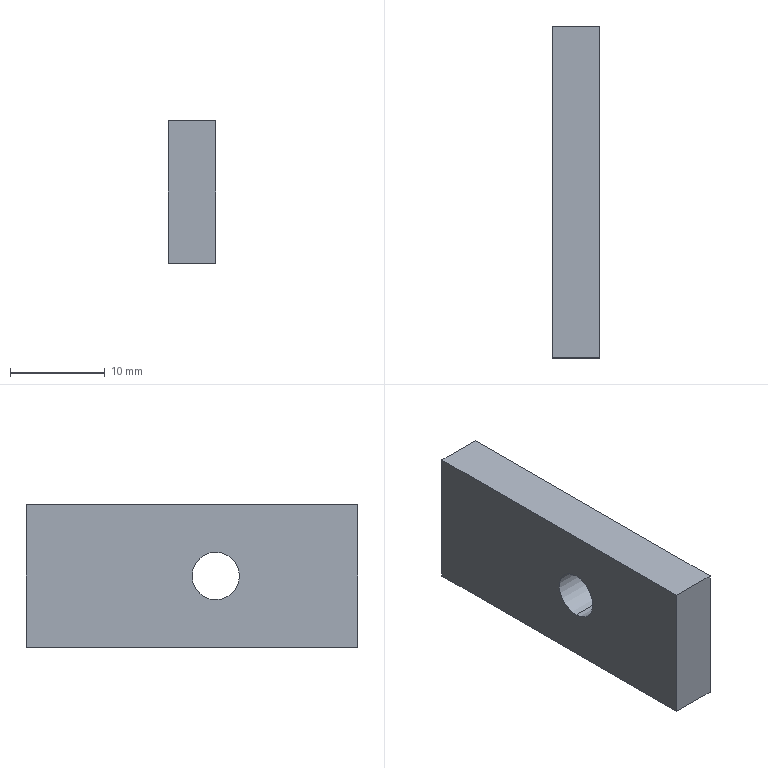Part | SolidWorks | features MBimport 1 | 1 solid | 8 faces | box 5 x 35 x 15 mm | volume 2527 mm3 | plane 6 | cylinder 2 | commonest cylinder face diameters 5 x2
STEP:
#1=CARTESIAN_POINT('',(0.,-15.,7.5));
#2=VERTEX_POINT('',#1);
#3=CARTESIAN_POINT('',(0.,-15.,-7.5));
#4=VERTEX_POINT('',#3);
#5=CARTESIAN_POINT('',(0.,-15.,7.5));
#6=DIRECTION('',(0.,0.,-1.));
#7=VECTOR('',#6,1000.);
#8=LINE('',#5,#7);
#9=EDGE_CURVE('',#2,#4,#8,.T.);
#10=ORIENTED_EDGE('',*,*,#9,.F.);
#11=CARTESIAN_POINT('',(0.,20.,7.5));
#12=VERTEX_POINT('',#11);
#13=CARTESIAN_POINT('',(0.,-15.,7.5));
#14=DIRECTION('',(0.,1.,0.));
#15=VECTOR('',#14,1000.);
#16=LINE('',#13,#15);
#17=EDGE_CURVE('',#2,#12,#16,.T.);
#18=ORIENTED_EDGE('',*,*,#17,.T.);
#19=CARTESIAN_POINT('',(0.,20.,-7.5));
#20=VERTEX_POINT('',#19);
#21=CARTESIAN_POINT('',(0.,20.,-7.5));
#22=DIRECTION('',(0.,0.,1.));
#23=VECTOR('',#22,1000.);
#24=LINE('',#21,#23);
#25=EDGE_CURVE('',#20,#12,#24,.T.);
#26=ORIENTED_EDGE('',*,*,#25,.F.);
#27=CARTESIAN_POINT('',(0.,20.,-7.5));
#28=DIRECTION('',(0.,-1.,0.));
#29=VECTOR('',#28,1000.);
#30=LINE('',#27,#29);
#31=EDGE_CURVE('',#20,#4,#30,.T.);
#32=ORIENTED_EDGE('',*,*,#31,.T.);
#33=EDGE_LOOP('',(#10,#18,#26,#32));
#34=FACE_OUTER_BOUND('',#33,.T.);
#35=CARTESIAN_POINT('',(0.,0.,2.5));
#36=VERTEX_POINT('',#35);
#37=CARTESIAN_POINT('',(0.,0.,-2.5));
#38=VERTEX_POINT('',#37);
#39=CARTESIAN_POINT('',(0.,0.,0.));
#40=DIRECTION('',(1.,0.,0.));
#41=DIRECTION('',(0.,0.,1.));
#42=AXIS2_PLACEMENT_3D('',#39,#40,#41);
#43=CIRCLE('',#42,2.5);
#44=EDGE_CURVE('',#36,#38,#43,.T.);
#45=ORIENTED_EDGE('',*,*,#44,.T.);
#46=CARTESIAN_POINT('',(0.,0.,0.));
#47=DIRECTION('',(1.,0.,0.));
#48=DIRECTION('',(0.,0.,-1.));
#49=AXIS2_PLACEMENT_3D('',#46,#47,#48);
#50=CIRCLE('',#49,2.5);
#51=EDGE_CURVE('',#38,#36,#50,.T.);
#52=ORIENTED_EDGE('',*,*,#51,.T.);
#53=EDGE_LOOP('',(#45,#52));
#54=FACE_BOUND('',#53,.T.);
#55=CARTESIAN_POINT('',(0.,0.,0.));
#56=DIRECTION('',(1.,0.,0.));
#57=DIRECTION('',(0.,1.,0.));
#58=AXIS2_PLACEMENT_3D('',#55,#56,#57);
#59=PLANE('',#58);
#60=ADVANCED_FACE('',(#34,#54),#59,.F.);
#61=CARTESIAN_POINT('',(5.,-15.,-7.5));
#62=VERTEX_POINT('',#61);
#63=CARTESIAN_POINT('',(0.,-15.,-7.5));
#64=DIRECTION('',(1.,0.,0.));
#65=VECTOR('',#64,1000.);
#66=LINE('',#63,#65);
#67=EDGE_CURVE('',#4,#62,#66,.T.);
#68=ORIENTED_EDGE('',*,*,#67,.T.);
#69=CARTESIAN_POINT('',(5.,-15.,7.5));
#70=VERTEX_POINT('',#69);
#71=CARTESIAN_POINT('',(5.,-15.,7.5));
#72=DIRECTION('',(0.,0.,-1.));
#73=VECTOR('',#72,1000.);
#74=LINE('',#71,#73);
#75=EDGE_CURVE('',#70,#62,#74,.T.);
#76=ORIENTED_EDGE('',*,*,#75,.F.);
#77=CARTESIAN_POINT('',(0.,-15.,7.5));
#78=DIRECTION('',(1.,0.,0.));
#79=VECTOR('',#78,1000.);
#80=LINE('',#77,#79);
#81=EDGE_CURVE('',#2,#70,#80,.T.);
#82=ORIENTED_EDGE('',*,*,#81,.F.);
#83=ORIENTED_EDGE('',*,*,#9,.T.);
#84=EDGE_LOOP('',(#68,#76,#82,#83));
#85=FACE_OUTER_BOUND('',#84,.T.);
#86=CARTESIAN_POINT('',(0.,-15.,7.5));
#87=DIRECTION('',(0.,-1.,0.));
#88=DIRECTION('',(0.,0.,-1.));
#89=AXIS2_PLACEMENT_3D('',#86,#87,#88);
#90=PLANE('',#89);
#91=ADVANCED_FACE('',(#85),#90,.T.);
#92=ORIENTED_EDGE('',*,*,#81,.T.);
#93=CARTESIAN_POINT('',(5.,20.,7.5));
#94=VERTEX_POINT('',#93);
#95=CARTESIAN_POINT('',(5.,-15.,7.5));
#96=DIRECTION('',(0.,1.,0.));
#97=VECTOR('',#96,1000.);
#98=LINE('',#95,#97);
#99=EDGE_CURVE('',#70,#94,#98,.T.);
#100=ORIENTED_EDGE('',*,*,#99,.T.);
#101=CARTESIAN_POINT('',(0.,20.,7.5));
#102=DIRECTION('',(1.,0.,0.));
#103=VECTOR('',#102,1000.);
#104=LINE('',#101,#103);
#105=EDGE_CURVE('',#12,#94,#104,.T.);
#106=ORIENTED_EDGE('',*,*,#105,.F.);
#107=ORIENTED_EDGE('',*,*,#17,.F.);
#108=EDGE_LOOP('',(#92,#100,#106,#107));
#109=FACE_OUTER_BOUND('',#108,.T.);
#110=CARTESIAN_POINT('',(0.,15.,7.5));
#111=DIRECTION('',(0.,0.,1.));
#112=DIRECTION('',(0.,-1.,0.));
#113=AXIS2_PLACEMENT_3D('',#110,#111,#112);
#114=PLANE('',#113);
#115=ADVANCED_FACE('',(#109),#114,.T.);
#116=ORIENTED_EDGE('',*,*,#105,.T.);
#117=CARTESIAN_POINT('',(5.,20.,-7.5));
#118=VERTEX_POINT('',#117);
#119=CARTESIAN_POINT('',(5.,20.,7.5));
#120=DIRECTION('',(0.,0.,-1.));
#121=VECTOR('',#120,1000.);
#122=LINE('',#119,#121);
#123=EDGE_CURVE('',#94,#118,#122,.T.);
#124=ORIENTED_EDGE('',*,*,#123,.T.);
#125=CARTESIAN_POINT('',(5.,20.,-7.5));
#126=DIRECTION('',(-1.,0.,0.));
#127=VECTOR('',#126,1000.);
#128=LINE('',#125,#127);
#129=EDGE_CURVE('',#118,#20,#128,.T.);
#130=ORIENTED_EDGE('',*,*,#129,.T.);
#131=ORIENTED_EDGE('',*,*,#25,.T.);
#132=EDGE_LOOP('',(#116,#124,#130,#131));
#133=FACE_OUTER_BOUND('',#132,.T.);
#134=CARTESIAN_POINT('',(0.,20.,0.));
#135=DIRECTION('',(0.,1.,0.));
#136=DIRECTION('',(0.,0.,1.));
#137=AXIS2_PLACEMENT_3D('',#134,#135,#136);
#138=PLANE('',#137);
#139=ADVANCED_FACE('',(#133),#138,.T.);
#140=ORIENTED_EDGE('',*,*,#67,.F.);
#141=ORIENTED_EDGE('',*,*,#31,.F.);
#142=ORIENTED_EDGE('',*,*,#129,.F.);
#143=CARTESIAN_POINT('',(5.,-15.,-7.5));
#144=DIRECTION('',(0.,1.,0.));
#145=VECTOR('',#144,1000.);
#146=LINE('',#143,#145);
#147=EDGE_CURVE('',#62,#118,#146,.T.);
#148=ORIENTED_EDGE('',*,*,#147,.F.);
#149=EDGE_LOOP('',(#140,#141,#142,#148));
#150=FACE_OUTER_BOUND('',#149,.T.);
#151=CARTESIAN_POINT('',(0.,-15.,-7.5));
#152=DIRECTION('',(0.,0.,-1.));
#153=DIRECTION('',(0.,1.,0.));
#154=AXIS2_PLACEMENT_3D('',#151,#152,#153);
#155=PLANE('',#154);
#156=ADVANCED_FACE('',(#150),#155,.T.);
#157=CARTESIAN_POINT('',(5.,0.,2.5));
#158=VERTEX_POINT('',#157);
#159=CARTESIAN_POINT('',(5.,0.,2.5));
#160=DIRECTION('',(-1.,0.,0.));
#161=VECTOR('',#160,1000.);
#162=LINE('',#159,#161);
#163=EDGE_CURVE('',#158,#36,#162,.T.);
#164=ORIENTED_EDGE('',*,*,#163,.F.);
#165=CARTESIAN_POINT('',(5.,0.,-2.5));
#166=VERTEX_POINT('',#165);
#167=CARTESIAN_POINT('',(5.,0.,0.));
#168=DIRECTION('',(1.,0.,0.));
#169=DIRECTION('',(0.,0.,1.));
#170=AXIS2_PLACEMENT_3D('',#167,#168,#169);
#171=CIRCLE('',#170,2.5);
#172=EDGE_CURVE('',#158,#166,#171,.T.);
#173=ORIENTED_EDGE('',*,*,#172,.T.);
#174=CARTESIAN_POINT('',(5.,0.,-2.5));
#175=DIRECTION('',(-1.,0.,0.));
#176=VECTOR('',#175,1000.);
#177=LINE('',#174,#176);
#178=EDGE_CURVE('',#166,#38,#177,.T.);
#179=ORIENTED_EDGE('',*,*,#178,.T.);
#180=ORIENTED_EDGE('',*,*,#44,.F.);
#181=EDGE_LOOP('',(#164,#173,#179,#180));
#182=FACE_OUTER_BOUND('',#181,.T.);
#183=CARTESIAN_POINT('',(5.,0.,0.));
#184=DIRECTION('',(-1.,0.,0.));
#185=DIRECTION('',(0.,0.,-1.));
#186=AXIS2_PLACEMENT_3D('',#183,#184,#185);
#187=CYLINDRICAL_SURFACE('',#186,2.5);
#188=ADVANCED_FACE('',(#182),#187,.F.);
#189=ORIENTED_EDGE('',*,*,#178,.F.);
#190=CARTESIAN_POINT('',(5.,0.,0.));
#191=DIRECTION('',(1.,0.,0.));
#192=DIRECTION('',(0.,0.,-1.));
#193=AXIS2_PLACEMENT_3D('',#190,#191,#192);
#194=CIRCLE('',#193,2.5);
#195=EDGE_CURVE('',#166,#158,#194,.T.);
#196=ORIENTED_EDGE('',*,*,#195,.T.);
#197=ORIENTED_EDGE('',*,*,#163,.T.);
#198=ORIENTED_EDGE('',*,*,#51,.F.);
#199=EDGE_LOOP('',(#189,#196,#197,#198));
#200=FACE_OUTER_BOUND('',#199,.T.);
#201=CARTESIAN_POINT('',(5.,0.,0.));
#202=DIRECTION('',(-1.,0.,0.));
#203=DIRECTION('',(0.,0.,-1.));
#204=AXIS2_PLACEMENT_3D('',#201,#202,#203);
#205=CYLINDRICAL_SURFACE('',#204,2.5);
#206=ADVANCED_FACE('',(#200),#205,.F.);
#207=ORIENTED_EDGE('',*,*,#75,.T.);
#208=ORIENTED_EDGE('',*,*,#147,.T.);
#209=ORIENTED_EDGE('',*,*,#123,.F.);
#210=ORIENTED_EDGE('',*,*,#99,.F.);
#211=EDGE_LOOP('',(#207,#208,#209,#210));
#212=FACE_OUTER_BOUND('',#211,.T.);
#213=ORIENTED_EDGE('',*,*,#172,.F.);
#214=ORIENTED_EDGE('',*,*,#195,.F.);
#215=EDGE_LOOP('',(#213,#214));
#216=FACE_BOUND('',#215,.T.);
#217=CARTESIAN_POINT('',(5.,0.,0.));
#218=DIRECTION('',(1.,0.,0.));
#219=DIRECTION('',(0.,1.,0.));
#220=AXIS2_PLACEMENT_3D('',#217,#218,#219);
#221=PLANE('',#220);
#222=ADVANCED_FACE('',(#212,#216),#221,.T.);
#223=CLOSED_SHELL('',(#60,#91,#115,#139,#156,#188,#206,#222));
#224=MANIFOLD_SOLID_BREP('',#223);
#225=CARTESIAN_POINT('',(0.,0.,0.));
#226=DIRECTION('',(0.,0.,1.));
#227=DIRECTION('',(1.,0.,0.));
#228=AXIS2_PLACEMENT_3D('',#225,#226,#227);
#229=(LENGTH_UNIT()NAMED_UNIT(*)SI_UNIT(.MILLI.,.METRE.));
#230=UNCERTAINTY_MEASURE_WITH_UNIT(LENGTH_MEASURE(0.00001),#229,'','');
#231=(NAMED_UNIT(*)PLANE_ANGLE_UNIT()SI_UNIT($,.RADIAN.));
#232=(NAMED_UNIT(*)SI_UNIT($,.STERADIAN.)SOLID_ANGLE_UNIT());
#233=(GEOMETRIC_REPRESENTATION_CONTEXT(3)GLOBAL_UNCERTAINTY_ASSIGNED_CONTEXT((#230))GLOBAL_UNIT_ASSIGNED_CONTEXT((#229,#231,#232))REPRESENTATION_CONTEXT('',''));
#234=ADVANCED_BREP_SHAPE_REPRESENTATION('',(#224,#228),#233);